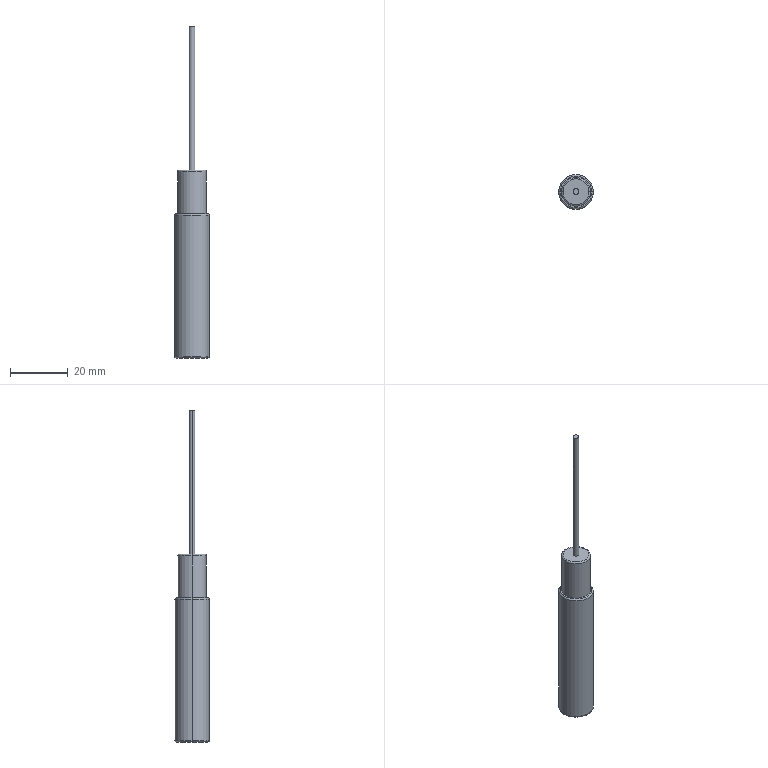Part | STEP file | YB Inductive Proximity Switch | 1 solid | 16 faces | box 12 x 12 x 115 mm | volume 6984 mm3 | torus 6 | cylinder 6 | plane 4 | commonest cylinder face diameters 2 x2 10 x2 12 x2
STEP:
#1=CARTESIAN_POINT('',(0.,0.,0.));
#2=DIRECTION('',(0.,0.,1.));
#3=DIRECTION('',(1.,0.,0.));
#4=AXIS2_PLACEMENT_3D('',#1,#2,#3);
#5=CARTESIAN_POINT('',(-5.5,0.,0.));
#6=VERTEX_POINT('',#5);
#7=CARTESIAN_POINT('',(5.5,0.,0.));
#8=VERTEX_POINT('',#7);
#9=CARTESIAN_POINT('',(0.,0.,0.));
#10=DIRECTION('',(0.,0.,-1.));
#11=DIRECTION('',(1.,0.,0.));
#12=AXIS2_PLACEMENT_3D('',#9,#10,#11);
#13=CIRCLE('',#12,5.5);
#14=CARTESIAN_POINT('',(0.,0.,0.5));
#15=DIRECTION('',(0.,0.,1.));
#16=DIRECTION('',(1.,0.,0.));
#17=AXIS2_PLACEMENT_3D('',#14,#15,#16);
#18=TOROIDAL_SURFACE('',#17,5.5,0.5);
#19=CARTESIAN_POINT('',(6.283,4.712));
#20=DIRECTION('',(-1.,0.));
#21=VECTOR('',#20,1.);
#22=LINE('',#19,#21);
#23=(GEOMETRIC_REPRESENTATION_CONTEXT(2)PARAMETRIC_REPRESENTATION_CONTEXT()REPRESENTATION_CONTEXT('',''));
#24=DEFINITIONAL_REPRESENTATION('',(#22),#23);
#25=PCURVE('',#18,#24);
#26=CARTESIAN_POINT('',(0.,0.,0.));
#27=DIRECTION('',(0.,0.,1.));
#28=DIRECTION('',(1.,0.,0.));
#29=AXIS2_PLACEMENT_3D('',#26,#27,#28);
#30=PLANE('',#29);
#31=CARTESIAN_POINT('',(5.5,0.));
#32=CARTESIAN_POINT('',(5.5,-9.526));
#33=CARTESIAN_POINT('',(-2.75,-4.763));
#34=CARTESIAN_POINT('',(-11.,0.));
#35=CARTESIAN_POINT('',(-2.75,4.763));
#36=CARTESIAN_POINT('',(5.5,9.526));
#37=CARTESIAN_POINT('',(5.5,0.));
#38=(BOUNDED_CURVE()B_SPLINE_CURVE(2,(#31,#32,#33,#34,#35,#36,#37),.UNSPECIFIED.,.T.,.F.)B_SPLINE_CURVE_WITH_KNOTS((1,2,2,2,2,1),(-2.094,0.,2.094,4.189,6.283,8.378),.UNSPECIFIED.)CURVE()GEOMETRIC_REPRESENTATION_ITEM()RATIONAL_B_SPLINE_CURVE((1.,0.5,1.,0.5,1.,0.5,1.))REPRESENTATION_ITEM(''));
#39=(GEOMETRIC_REPRESENTATION_CONTEXT(2)PARAMETRIC_REPRESENTATION_CONTEXT()REPRESENTATION_CONTEXT('',''));
#40=DEFINITIONAL_REPRESENTATION('',(#38),#39);
#41=PCURVE('',#30,#40);
#42=SURFACE_CURVE('',#13,(#25,#41),.PCURVE_S1.);
#43=EDGE_CURVE('',#6,#8,#42,.T.);
#44=ORIENTED_EDGE('',*,*,#43,.F.);
#45=CARTESIAN_POINT('',(-6.,0.,0.5));
#46=VERTEX_POINT('',#45);
#47=CARTESIAN_POINT('',(-5.5,0.,0.5));
#48=DIRECTION('',(0.,1.,0.));
#49=DIRECTION('',(-1.,0.,0.));
#50=AXIS2_PLACEMENT_3D('',#47,#48,#49);
#51=CIRCLE('',#50,0.5);
#52=CARTESIAN_POINT('',(3.142,0.));
#53=DIRECTION('',(0.,1.));
#54=VECTOR('',#53,1.);
#55=LINE('',#52,#54);
#56=(GEOMETRIC_REPRESENTATION_CONTEXT(2)PARAMETRIC_REPRESENTATION_CONTEXT()REPRESENTATION_CONTEXT('',''));
#57=DEFINITIONAL_REPRESENTATION('',(#55),#56);
#58=PCURVE('',#18,#57);
#59=CARTESIAN_POINT('',(0.,0.,0.5));
#60=DIRECTION('',(0.,0.,1.));
#61=DIRECTION('',(1.,0.,0.));
#62=AXIS2_PLACEMENT_3D('',#59,#60,#61);
#63=TOROIDAL_SURFACE('',#62,5.5,0.5);
#64=CARTESIAN_POINT('',(3.142,0.));
#65=DIRECTION('',(0.,1.));
#66=VECTOR('',#65,1.);
#67=LINE('',#64,#66);
#68=(GEOMETRIC_REPRESENTATION_CONTEXT(2)PARAMETRIC_REPRESENTATION_CONTEXT()REPRESENTATION_CONTEXT('',''));
#69=DEFINITIONAL_REPRESENTATION('',(#67),#68);
#70=PCURVE('',#63,#69);
#71=SURFACE_CURVE('',#51,(#58,#70),.PCURVE_S1.);
#72=EDGE_CURVE('',#6,#46,#71,.T.);
#73=ORIENTED_EDGE('',*,*,#72,.T.);
#74=CARTESIAN_POINT('',(6.,0.,0.5));
#75=VERTEX_POINT('',#74);
#76=CARTESIAN_POINT('',(0.,0.,0.5));
#77=DIRECTION('',(0.,0.,1.));
#78=DIRECTION('',(1.,0.,0.));
#79=AXIS2_PLACEMENT_3D('',#76,#77,#78);
#80=CIRCLE('',#79,6.);
#81=CARTESIAN_POINT('',(0.,6.283));
#82=DIRECTION('',(1.,0.));
#83=VECTOR('',#82,1.);
#84=LINE('',#81,#83);
#85=(GEOMETRIC_REPRESENTATION_CONTEXT(2)PARAMETRIC_REPRESENTATION_CONTEXT()REPRESENTATION_CONTEXT('',''));
#86=DEFINITIONAL_REPRESENTATION('',(#84),#85);
#87=PCURVE('',#18,#86);
#88=CARTESIAN_POINT('',(0.,0.,50.));
#89=DIRECTION('',(0.,0.,-1.));
#90=DIRECTION('',(-1.,0.,0.));
#91=AXIS2_PLACEMENT_3D('',#88,#89,#90);
#92=CYLINDRICAL_SURFACE('',#91,6.);
#93=CARTESIAN_POINT('',(3.142,49.5));
#94=DIRECTION('',(-1.,0.));
#95=VECTOR('',#94,1.);
#96=LINE('',#93,#95);
#97=(GEOMETRIC_REPRESENTATION_CONTEXT(2)PARAMETRIC_REPRESENTATION_CONTEXT()REPRESENTATION_CONTEXT('',''));
#98=DEFINITIONAL_REPRESENTATION('',(#96),#97);
#99=PCURVE('',#92,#98);
#100=SURFACE_CURVE('',#80,(#87,#99),.PCURVE_S1.);
#101=EDGE_CURVE('',#75,#46,#100,.T.);
#102=ORIENTED_EDGE('',*,*,#101,.F.);
#103=CARTESIAN_POINT('',(5.5,0.,0.5));
#104=DIRECTION('',(0.,-1.,0.));
#105=DIRECTION('',(0.,0.,-1.));
#106=AXIS2_PLACEMENT_3D('',#103,#104,#105);
#107=CIRCLE('',#106,0.5);
#108=CARTESIAN_POINT('',(0.,4.712));
#109=DIRECTION('',(0.,1.));
#110=VECTOR('',#109,1.);
#111=LINE('',#108,#110);
#112=(GEOMETRIC_REPRESENTATION_CONTEXT(2)PARAMETRIC_REPRESENTATION_CONTEXT()REPRESENTATION_CONTEXT('',''));
#113=DEFINITIONAL_REPRESENTATION('',(#111),#112);
#114=PCURVE('',#18,#113);
#115=CARTESIAN_POINT('',(6.283,4.712));
#116=DIRECTION('',(0.,1.));
#117=VECTOR('',#116,1.);
#118=LINE('',#115,#117);
#119=(GEOMETRIC_REPRESENTATION_CONTEXT(2)PARAMETRIC_REPRESENTATION_CONTEXT()REPRESENTATION_CONTEXT('',''));
#120=DEFINITIONAL_REPRESENTATION('',(#118),#119);
#121=PCURVE('',#63,#120);
#122=SURFACE_CURVE('',#107,(#114,#121),.PCURVE_S1.);
#123=EDGE_CURVE('',#8,#75,#122,.T.);
#124=ORIENTED_EDGE('',*,*,#123,.F.);
#125=EDGE_LOOP('',(#44,#73,#102,#124));
#126=FACE_BOUND('',#125,.T.);
#127=ADVANCED_FACE('',(#126),#18,.T.);
#128=CARTESIAN_POINT('',(-6.,0.,49.5));
#129=VERTEX_POINT('',#128);
#130=CARTESIAN_POINT('',(6.,0.,49.5));
#131=VERTEX_POINT('',#130);
#132=CARTESIAN_POINT('',(0.,0.,49.5));
#133=DIRECTION('',(0.,0.,-1.));
#134=DIRECTION('',(1.,0.,0.));
#135=AXIS2_PLACEMENT_3D('',#132,#133,#134);
#136=CIRCLE('',#135,6.);
#137=CARTESIAN_POINT('',(0.,0.,49.5));
#138=DIRECTION('',(0.,0.,1.));
#139=DIRECTION('',(1.,0.,0.));
#140=AXIS2_PLACEMENT_3D('',#137,#138,#139);
#141=TOROIDAL_SURFACE('',#140,5.5,0.5);
#142=CARTESIAN_POINT('',(6.283,0.));
#143=DIRECTION('',(-1.,0.));
#144=VECTOR('',#143,1.);
#145=LINE('',#142,#144);
#146=(GEOMETRIC_REPRESENTATION_CONTEXT(2)PARAMETRIC_REPRESENTATION_CONTEXT()REPRESENTATION_CONTEXT('',''));
#147=DEFINITIONAL_REPRESENTATION('',(#145),#146);
#148=PCURVE('',#141,#147);
#149=CARTESIAN_POINT('',(-3.142,0.5));
#150=DIRECTION('',(1.,0.));
#151=VECTOR('',#150,1.);
#152=LINE('',#149,#151);
#153=(GEOMETRIC_REPRESENTATION_CONTEXT(2)PARAMETRIC_REPRESENTATION_CONTEXT()REPRESENTATION_CONTEXT('',''));
#154=DEFINITIONAL_REPRESENTATION('',(#152),#153);
#155=PCURVE('',#92,#154);
#156=SURFACE_CURVE('',#136,(#148,#155),.PCURVE_S1.);
#157=EDGE_CURVE('',#129,#131,#156,.T.);
#158=ORIENTED_EDGE('',*,*,#157,.F.);
#159=CARTESIAN_POINT('',(-5.5,0.,50.));
#160=VERTEX_POINT('',#159);
#161=CARTESIAN_POINT('',(-5.5,0.,49.5));
#162=DIRECTION('',(0.,1.,0.));
#163=DIRECTION('',(-1.,0.,0.));
#164=AXIS2_PLACEMENT_3D('',#161,#162,#163);
#165=CIRCLE('',#164,0.5);
#166=CARTESIAN_POINT('',(3.142,0.));
#167=DIRECTION('',(0.,1.));
#168=VECTOR('',#167,1.);
#169=LINE('',#166,#168);
#170=(GEOMETRIC_REPRESENTATION_CONTEXT(2)PARAMETRIC_REPRESENTATION_CONTEXT()REPRESENTATION_CONTEXT('',''));
#171=DEFINITIONAL_REPRESENTATION('',(#169),#170);
#172=PCURVE('',#141,#171);
#173=CARTESIAN_POINT('',(0.,0.,49.5));
#174=DIRECTION('',(0.,0.,1.));
#175=DIRECTION('',(1.,0.,0.));
#176=AXIS2_PLACEMENT_3D('',#173,#174,#175);
#177=TOROIDAL_SURFACE('',#176,5.5,0.5);
#178=CARTESIAN_POINT('',(3.142,0.));
#179=DIRECTION('',(0.,1.));
#180=VECTOR('',#179,1.);
#181=LINE('',#178,#180);
#182=(GEOMETRIC_REPRESENTATION_CONTEXT(2)PARAMETRIC_REPRESENTATION_CONTEXT()REPRESENTATION_CONTEXT('',''));
#183=DEFINITIONAL_REPRESENTATION('',(#181),#182);
#184=PCURVE('',#177,#183);
#185=SURFACE_CURVE('',#165,(#172,#184),.PCURVE_S1.);
#186=EDGE_CURVE('',#129,#160,#185,.T.);
#187=ORIENTED_EDGE('',*,*,#186,.T.);
#188=CARTESIAN_POINT('',(5.5,0.,50.));
#189=VERTEX_POINT('',#188);
#190=CARTESIAN_POINT('',(0.,0.,50.));
#191=DIRECTION('',(0.,0.,1.));
#192=DIRECTION('',(1.,0.,0.));
#193=AXIS2_PLACEMENT_3D('',#190,#191,#192);
#194=CIRCLE('',#193,5.5);
#195=CARTESIAN_POINT('',(0.,1.571));
#196=DIRECTION('',(1.,0.));
#197=VECTOR('',#196,1.);
#198=LINE('',#195,#197);
#199=(GEOMETRIC_REPRESENTATION_CONTEXT(2)PARAMETRIC_REPRESENTATION_CONTEXT()REPRESENTATION_CONTEXT('',''));
#200=DEFINITIONAL_REPRESENTATION('',(#198),#199);
#201=PCURVE('',#141,#200);
#202=CARTESIAN_POINT('',(0.,0.,50.));
#203=DIRECTION('',(0.,0.,1.));
#204=DIRECTION('',(1.,0.,0.));
#205=AXIS2_PLACEMENT_3D('',#202,#203,#204);
#206=PLANE('',#205);
#207=CARTESIAN_POINT('',(0.,0.));
#208=DIRECTION('',(1.,0.));
#209=AXIS2_PLACEMENT_2D('',#207,#208);
#210=CIRCLE('',#209,5.5);
#211=(GEOMETRIC_REPRESENTATION_CONTEXT(2)PARAMETRIC_REPRESENTATION_CONTEXT()REPRESENTATION_CONTEXT('',''));
#212=DEFINITIONAL_REPRESENTATION('',(#210),#211);
#213=PCURVE('',#206,#212);
#214=SURFACE_CURVE('',#194,(#201,#213),.PCURVE_S1.);
#215=EDGE_CURVE('',#189,#160,#214,.T.);
#216=ORIENTED_EDGE('',*,*,#215,.F.);
#217=CARTESIAN_POINT('',(5.5,0.,49.5));
#218=DIRECTION('',(0.,-1.,0.));
#219=DIRECTION('',(0.,0.,-1.));
#220=AXIS2_PLACEMENT_3D('',#217,#218,#219);
#221=CIRCLE('',#220,0.5);
#222=CARTESIAN_POINT('',(0.,-1.571));
#223=DIRECTION('',(0.,1.));
#224=VECTOR('',#223,1.);
#225=LINE('',#222,#224);
#226=(GEOMETRIC_REPRESENTATION_CONTEXT(2)PARAMETRIC_REPRESENTATION_CONTEXT()REPRESENTATION_CONTEXT('',''));
#227=DEFINITIONAL_REPRESENTATION('',(#225),#226);
#228=PCURVE('',#141,#227);
#229=CARTESIAN_POINT('',(6.283,-1.571));
#230=DIRECTION('',(0.,1.));
#231=VECTOR('',#230,1.);
#232=LINE('',#229,#231);
#233=(GEOMETRIC_REPRESENTATION_CONTEXT(2)PARAMETRIC_REPRESENTATION_CONTEXT()REPRESENTATION_CONTEXT('',''));
#234=DEFINITIONAL_REPRESENTATION('',(#232),#233);
#235=PCURVE('',#177,#234);
#236=SURFACE_CURVE('',#221,(#228,#235),.PCURVE_S1.);
#237=EDGE_CURVE('',#131,#189,#236,.T.);
#238=ORIENTED_EDGE('',*,*,#237,.F.);
#239=EDGE_LOOP('',(#158,#187,#216,#238));
#240=FACE_BOUND('',#239,.T.);
#241=ADVANCED_FACE('',(#240),#141,.T.);
#242=CARTESIAN_POINT('',(-5.,0.,64.5));
#243=VERTEX_POINT('',#242);
#244=CARTESIAN_POINT('',(5.,0.,64.5));
#245=VERTEX_POINT('',#244);
#246=CARTESIAN_POINT('',(0.,0.,64.5));
#247=DIRECTION('',(0.,0.,-1.));
#248=DIRECTION('',(1.,0.,0.));
#249=AXIS2_PLACEMENT_3D('',#246,#247,#248);
#250=CIRCLE('',#249,5.);
#251=CARTESIAN_POINT('',(0.,0.,64.5));
#252=DIRECTION('',(0.,0.,1.));
#253=DIRECTION('',(1.,0.,0.));
#254=AXIS2_PLACEMENT_3D('',#251,#252,#253);
#255=TOROIDAL_SURFACE('',#254,4.5,0.5);
#256=CARTESIAN_POINT('',(6.283,0.));
#257=DIRECTION('',(-1.,0.));
#258=VECTOR('',#257,1.);
#259=LINE('',#256,#258);
#260=(GEOMETRIC_REPRESENTATION_CONTEXT(2)PARAMETRIC_REPRESENTATION_CONTEXT()REPRESENTATION_CONTEXT('',''));
#261=DEFINITIONAL_REPRESENTATION('',(#259),#260);
#262=PCURVE('',#255,#261);
#263=CARTESIAN_POINT('',(0.,0.,65.));
#264=DIRECTION('',(0.,0.,-1.));
#265=DIRECTION('',(-1.,0.,0.));
#266=AXIS2_PLACEMENT_3D('',#263,#264,#265);
#267=CYLINDRICAL_SURFACE('',#266,5.);
#268=CARTESIAN_POINT('',(-3.142,0.5));
#269=DIRECTION('',(1.,0.));
#270=VECTOR('',#269,1.);
#271=LINE('',#268,#270);
#272=(GEOMETRIC_REPRESENTATION_CONTEXT(2)PARAMETRIC_REPRESENTATION_CONTEXT()REPRESENTATION_CONTEXT('',''));
#273=DEFINITIONAL_REPRESENTATION('',(#271),#272);
#274=PCURVE('',#267,#273);
#275=SURFACE_CURVE('',#250,(#262,#274),.PCURVE_S1.);
#276=EDGE_CURVE('',#243,#245,#275,.T.);
#277=ORIENTED_EDGE('',*,*,#276,.F.);
#278=CARTESIAN_POINT('',(-4.5,0.,65.));
#279=VERTEX_POINT('',#278);
#280=CARTESIAN_POINT('',(-4.5,0.,64.5));
#281=DIRECTION('',(0.,1.,0.));
#282=DIRECTION('',(-1.,0.,0.));
#283=AXIS2_PLACEMENT_3D('',#280,#281,#282);
#284=CIRCLE('',#283,0.5);
#285=CARTESIAN_POINT('',(3.142,0.));
#286=DIRECTION('',(0.,1.));
#287=VECTOR('',#286,1.);
#288=LINE('',#285,#287);
#289=(GEOMETRIC_REPRESENTATION_CONTEXT(2)PARAMETRIC_REPRESENTATION_CONTEXT()REPRESENTATION_CONTEXT('',''));
#290=DEFINITIONAL_REPRESENTATION('',(#288),#289);
#291=PCURVE('',#255,#290);
#292=CARTESIAN_POINT('',(0.,0.,64.5));
#293=DIRECTION('',(0.,0.,1.));
#294=DIRECTION('',(1.,0.,0.));
#295=AXIS2_PLACEMENT_3D('',#292,#293,#294);
#296=TOROIDAL_SURFACE('',#295,4.5,0.5);
#297=CARTESIAN_POINT('',(3.142,0.));
#298=DIRECTION('',(0.,1.));
#299=VECTOR('',#298,1.);
#300=LINE('',#297,#299);
#301=(GEOMETRIC_REPRESENTATION_CONTEXT(2)PARAMETRIC_REPRESENTATION_CONTEXT()REPRESENTATION_CONTEXT('',''));
#302=DEFINITIONAL_REPRESENTATION('',(#300),#301);
#303=PCURVE('',#296,#302);
#304=SURFACE_CURVE('',#284,(#291,#303),.PCURVE_S1.);
#305=EDGE_CURVE('',#243,#279,#304,.T.);
#306=ORIENTED_EDGE('',*,*,#305,.T.);
#307=CARTESIAN_POINT('',(4.5,0.,65.));
#308=VERTEX_POINT('',#307);
#309=CARTESIAN_POINT('',(0.,0.,65.));
#310=DIRECTION('',(0.,0.,1.));
#311=DIRECTION('',(1.,0.,0.));
#312=AXIS2_PLACEMENT_3D('',#309,#310,#311);
#313=CIRCLE('',#312,4.5);
#314=CARTESIAN_POINT('',(0.,1.571));
#315=DIRECTION('',(1.,0.));
#316=VECTOR('',#315,1.);
#317=LINE('',#314,#316);
#318=(GEOMETRIC_REPRESENTATION_CONTEXT(2)PARAMETRIC_REPRESENTATION_CONTEXT()REPRESENTATION_CONTEXT('',''));
#319=DEFINITIONAL_REPRESENTATION('',(#317),#318);
#320=PCURVE('',#255,#319);
#321=CARTESIAN_POINT('',(0.,0.,65.));
#322=DIRECTION('',(0.,0.,1.));
#323=DIRECTION('',(1.,0.,0.));
#324=AXIS2_PLACEMENT_3D('',#321,#322,#323);
#325=PLANE('',#324);
#326=CARTESIAN_POINT('',(0.,0.));
#327=DIRECTION('',(1.,0.));
#328=AXIS2_PLACEMENT_2D('',#326,#327);
#329=CIRCLE('',#328,4.5);
#330=(GEOMETRIC_REPRESENTATION_CONTEXT(2)PARAMETRIC_REPRESENTATION_CONTEXT()REPRESENTATION_CONTEXT('',''));
#331=DEFINITIONAL_REPRESENTATION('',(#329),#330);
#332=PCURVE('',#325,#331);
#333=SURFACE_CURVE('',#313,(#320,#332),.PCURVE_S1.);
#334=EDGE_CURVE('',#308,#279,#333,.T.);
#335=ORIENTED_EDGE('',*,*,#334,.F.);
#336=CARTESIAN_POINT('',(4.5,0.,64.5));
#337=DIRECTION('',(0.,-1.,0.));
#338=DIRECTION('',(0.,0.,-1.));
#339=AXIS2_PLACEMENT_3D('',#336,#337,#338);
#340=CIRCLE('',#339,0.5);
#341=CARTESIAN_POINT('',(0.,-1.571));
#342=DIRECTION('',(0.,1.));
#343=VECTOR('',#342,1.);
#344=LINE('',#341,#343);
#345=(GEOMETRIC_REPRESENTATION_CONTEXT(2)PARAMETRIC_REPRESENTATION_CONTEXT()REPRESENTATION_CONTEXT('',''));
#346=DEFINITIONAL_REPRESENTATION('',(#344),#345);
#347=PCURVE('',#255,#346);
#348=CARTESIAN_POINT('',(6.283,-1.571));
#349=DIRECTION('',(0.,1.));
#350=VECTOR('',#349,1.);
#351=LINE('',#348,#350);
#352=(GEOMETRIC_REPRESENTATION_CONTEXT(2)PARAMETRIC_REPRESENTATION_CONTEXT()REPRESENTATION_CONTEXT('',''));
#353=DEFINITIONAL_REPRESENTATION('',(#351),#352);
#354=PCURVE('',#296,#353);
#355=SURFACE_CURVE('',#340,(#347,#354),.PCURVE_S1.);
#356=EDGE_CURVE('',#245,#308,#355,.T.);
#357=ORIENTED_EDGE('',*,*,#356,.F.);
#358=EDGE_LOOP('',(#277,#306,#335,#357));
#359=FACE_BOUND('',#358,.T.);
#360=ADVANCED_FACE('',(#359),#255,.T.);
#361=CARTESIAN_POINT('',(1.,0.,115.));
#362=VERTEX_POINT('',#361);
#363=CARTESIAN_POINT('',(-1.,0.,115.));
#364=VERTEX_POINT('',#363);
#365=CARTESIAN_POINT('',(0.,0.,115.));
#366=DIRECTION('',(0.,0.,1.));
#367=DIRECTION('',(1.,0.,0.));
#368=AXIS2_PLACEMENT_3D('',#365,#366,#367);
#369=CIRCLE('',#368,1.);
#370=CARTESIAN_POINT('',(0.,0.,115.));
#371=DIRECTION('',(0.,0.,-1.));
#372=DIRECTION('',(-1.,0.,0.));
#373=AXIS2_PLACEMENT_3D('',#370,#371,#372);
#374=CYLINDRICAL_SURFACE('',#373,1.);
#375=CARTESIAN_POINT('',(3.142,0.));
#376=DIRECTION('',(-1.,0.));
#377=VECTOR('',#376,1.);
#378=LINE('',#375,#377);
#379=(GEOMETRIC_REPRESENTATION_CONTEXT(2)PARAMETRIC_REPRESENTATION_CONTEXT()REPRESENTATION_CONTEXT('',''));
#380=DEFINITIONAL_REPRESENTATION('',(#378),#379);
#381=PCURVE('',#374,#380);
#382=CARTESIAN_POINT('',(0.,0.,115.));
#383=DIRECTION('',(0.,0.,1.));
#384=DIRECTION('',(1.,0.,0.));
#385=AXIS2_PLACEMENT_3D('',#382,#383,#384);
#386=PLANE('',#385);
#387=CARTESIAN_POINT('',(0.,0.));
#388=DIRECTION('',(1.,0.));
#389=AXIS2_PLACEMENT_2D('',#387,#388);
#390=CIRCLE('',#389,1.);
#391=(GEOMETRIC_REPRESENTATION_CONTEXT(2)PARAMETRIC_REPRESENTATION_CONTEXT()REPRESENTATION_CONTEXT('',''));
#392=DEFINITIONAL_REPRESENTATION('',(#390),#391);
#393=PCURVE('',#386,#392);
#394=SURFACE_CURVE('',#369,(#381,#393),.PCURVE_S1.);
#395=EDGE_CURVE('',#362,#364,#394,.T.);
#396=ORIENTED_EDGE('',*,*,#395,.F.);
#397=CARTESIAN_POINT('',(1.,0.,65.));
#398=VERTEX_POINT('',#397);
#399=CARTESIAN_POINT('',(1.,0.,115.));
#400=DIRECTION('',(0.,0.,-1.));
#401=VECTOR('',#400,1.);
#402=LINE('',#399,#401);
#403=CARTESIAN_POINT('',(3.142,0.));
#404=DIRECTION('',(0.,1.));
#405=VECTOR('',#404,1.);
#406=LINE('',#403,#405);
#407=(GEOMETRIC_REPRESENTATION_CONTEXT(2)PARAMETRIC_REPRESENTATION_CONTEXT()REPRESENTATION_CONTEXT('',''));
#408=DEFINITIONAL_REPRESENTATION('',(#406),#407);
#409=PCURVE('',#374,#408);
#410=CARTESIAN_POINT('',(0.,0.,115.));
#411=DIRECTION('',(0.,0.,-1.));
#412=DIRECTION('',(-1.,0.,0.));
#413=AXIS2_PLACEMENT_3D('',#410,#411,#412);
#414=CYLINDRICAL_SURFACE('',#413,1.);
#415=CARTESIAN_POINT('',(3.142,0.));
#416=DIRECTION('',(0.,1.));
#417=VECTOR('',#416,1.);
#418=LINE('',#415,#417);
#419=(GEOMETRIC_REPRESENTATION_CONTEXT(2)PARAMETRIC_REPRESENTATION_CONTEXT()REPRESENTATION_CONTEXT('',''));
#420=DEFINITIONAL_REPRESENTATION('',(#418),#419);
#421=PCURVE('',#414,#420);
#422=SURFACE_CURVE('',#402,(#409,#421),.PCURVE_S1.);
#423=EDGE_CURVE('',#362,#398,#422,.T.);
#424=ORIENTED_EDGE('',*,*,#423,.T.);
#425=CARTESIAN_POINT('',(-1.,0.,65.));
#426=VERTEX_POINT('',#425);
#427=CARTESIAN_POINT('',(0.,0.,65.));
#428=DIRECTION('',(0.,0.,1.));
#429=DIRECTION('',(1.,0.,0.));
#430=AXIS2_PLACEMENT_3D('',#427,#428,#429);
#431=CIRCLE('',#430,1.);
#432=CARTESIAN_POINT('',(3.142,50.));
#433=DIRECTION('',(-1.,0.));
#434=VECTOR('',#433,1.);
#435=LINE('',#432,#434);
#436=(GEOMETRIC_REPRESENTATION_CONTEXT(2)PARAMETRIC_REPRESENTATION_CONTEXT()REPRESENTATION_CONTEXT('',''));
#437=DEFINITIONAL_REPRESENTATION('',(#435),#436);
#438=PCURVE('',#374,#437);
#439=CARTESIAN_POINT('',(0.,0.));
#440=DIRECTION('',(1.,0.));
#441=AXIS2_PLACEMENT_2D('',#439,#440);
#442=CIRCLE('',#441,1.);
#443=(GEOMETRIC_REPRESENTATION_CONTEXT(2)PARAMETRIC_REPRESENTATION_CONTEXT()REPRESENTATION_CONTEXT('',''));
#444=DEFINITIONAL_REPRESENTATION('',(#442),#443);
#445=PCURVE('',#325,#444);
#446=SURFACE_CURVE('',#431,(#438,#445),.PCURVE_S1.);
#447=EDGE_CURVE('',#398,#426,#446,.T.);
#448=ORIENTED_EDGE('',*,*,#447,.T.);
#449=CARTESIAN_POINT('',(-1.,0.,115.));
#450=DIRECTION('',(0.,0.,-1.));
#451=VECTOR('',#450,1.);
#452=LINE('',#449,#451);
#453=CARTESIAN_POINT('',(0.,0.));
#454=DIRECTION('',(0.,1.));
#455=VECTOR('',#454,1.);
#456=LINE('',#453,#455);
#457=(GEOMETRIC_REPRESENTATION_CONTEXT(2)PARAMETRIC_REPRESENTATION_CONTEXT()REPRESENTATION_CONTEXT('',''));
#458=DEFINITIONAL_REPRESENTATION('',(#456),#457);
#459=PCURVE('',#374,#458);
#460=CARTESIAN_POINT('',(6.283,0.));
#461=DIRECTION('',(0.,1.));
#462=VECTOR('',#461,1.);
#463=LINE('',#460,#462);
#464=(GEOMETRIC_REPRESENTATION_CONTEXT(2)PARAMETRIC_REPRESENTATION_CONTEXT()REPRESENTATION_CONTEXT('',''));
#465=DEFINITIONAL_REPRESENTATION('',(#463),#464);
#466=PCURVE('',#414,#465);
#467=SURFACE_CURVE('',#452,(#459,#466),.PCURVE_S1.);
#468=EDGE_CURVE('',#364,#426,#467,.T.);
#469=ORIENTED_EDGE('',*,*,#468,.F.);
#470=EDGE_LOOP('',(#396,#424,#448,#469));
#471=FACE_BOUND('',#470,.T.);
#472=ADVANCED_FACE('',(#471),#374,.T.);
#473=ORIENTED_EDGE('',*,*,#276,.T.);
#474=CARTESIAN_POINT('',(5.,0.,50.));
#475=VERTEX_POINT('',#474);
#476=CARTESIAN_POINT('',(5.,0.,65.));
#477=DIRECTION('',(0.,0.,-1.));
#478=VECTOR('',#477,1.);
#479=LINE('',#476,#478);
#480=CARTESIAN_POINT('',(3.142,0.));
#481=DIRECTION('',(0.,1.));
#482=VECTOR('',#481,1.);
#483=LINE('',#480,#482);
#484=(GEOMETRIC_REPRESENTATION_CONTEXT(2)PARAMETRIC_REPRESENTATION_CONTEXT()REPRESENTATION_CONTEXT('',''));
#485=DEFINITIONAL_REPRESENTATION('',(#483),#484);
#486=PCURVE('',#267,#485);
#487=CARTESIAN_POINT('',(0.,0.,65.));
#488=DIRECTION('',(0.,0.,-1.));
#489=DIRECTION('',(-1.,0.,0.));
#490=AXIS2_PLACEMENT_3D('',#487,#488,#489);
#491=CYLINDRICAL_SURFACE('',#490,5.);
#492=CARTESIAN_POINT('',(3.142,0.));
#493=DIRECTION('',(0.,1.));
#494=VECTOR('',#493,1.);
#495=LINE('',#492,#494);
#496=(GEOMETRIC_REPRESENTATION_CONTEXT(2)PARAMETRIC_REPRESENTATION_CONTEXT()REPRESENTATION_CONTEXT('',''));
#497=DEFINITIONAL_REPRESENTATION('',(#495),#496);
#498=PCURVE('',#491,#497);
#499=SURFACE_CURVE('',#479,(#486,#498),.PCURVE_S1.);
#500=EDGE_CURVE('',#245,#475,#499,.T.);
#501=ORIENTED_EDGE('',*,*,#500,.T.);
#502=CARTESIAN_POINT('',(-5.,0.,50.));
#503=VERTEX_POINT('',#502);
#504=CARTESIAN_POINT('',(0.,0.,50.));
#505=DIRECTION('',(0.,0.,1.));
#506=DIRECTION('',(1.,0.,0.));
#507=AXIS2_PLACEMENT_3D('',#504,#505,#506);
#508=CIRCLE('',#507,5.);
#509=CARTESIAN_POINT('',(3.142,15.));
#510=DIRECTION('',(-1.,0.));
#511=VECTOR('',#510,1.);
#512=LINE('',#509,#511);
#513=(GEOMETRIC_REPRESENTATION_CONTEXT(2)PARAMETRIC_REPRESENTATION_CONTEXT()REPRESENTATION_CONTEXT('',''));
#514=DEFINITIONAL_REPRESENTATION('',(#512),#513);
#515=PCURVE('',#267,#514);
#516=CARTESIAN_POINT('',(0.,0.));
#517=DIRECTION('',(1.,0.));
#518=AXIS2_PLACEMENT_2D('',#516,#517);
#519=CIRCLE('',#518,5.);
#520=(GEOMETRIC_REPRESENTATION_CONTEXT(2)PARAMETRIC_REPRESENTATION_CONTEXT()REPRESENTATION_CONTEXT('',''));
#521=DEFINITIONAL_REPRESENTATION('',(#519),#520);
#522=PCURVE('',#206,#521);
#523=SURFACE_CURVE('',#508,(#515,#522),.PCURVE_S1.);
#524=EDGE_CURVE('',#475,#503,#523,.T.);
#525=ORIENTED_EDGE('',*,*,#524,.T.);
#526=CARTESIAN_POINT('',(-5.,0.,65.));
#527=DIRECTION('',(0.,0.,-1.));
#528=VECTOR('',#527,1.);
#529=LINE('',#526,#528);
#530=CARTESIAN_POINT('',(0.,0.));
#531=DIRECTION('',(0.,1.));
#532=VECTOR('',#531,1.);
#533=LINE('',#530,#532);
#534=(GEOMETRIC_REPRESENTATION_CONTEXT(2)PARAMETRIC_REPRESENTATION_CONTEXT()REPRESENTATION_CONTEXT('',''));
#535=DEFINITIONAL_REPRESENTATION('',(#533),#534);
#536=PCURVE('',#267,#535);
#537=CARTESIAN_POINT('',(6.283,0.));
#538=DIRECTION('',(0.,1.));
#539=VECTOR('',#538,1.);
#540=LINE('',#537,#539);
#541=(GEOMETRIC_REPRESENTATION_CONTEXT(2)PARAMETRIC_REPRESENTATION_CONTEXT()REPRESENTATION_CONTEXT('',''));
#542=DEFINITIONAL_REPRESENTATION('',(#540),#541);
#543=PCURVE('',#491,#542);
#544=SURFACE_CURVE('',#529,(#536,#543),.PCURVE_S1.);
#545=EDGE_CURVE('',#243,#503,#544,.T.);
#546=ORIENTED_EDGE('',*,*,#545,.F.);
#547=EDGE_LOOP('',(#473,#501,#525,#546));
#548=FACE_BOUND('',#547,.T.);
#549=ADVANCED_FACE('',(#548),#267,.T.);
#550=ORIENTED_EDGE('',*,*,#157,.T.);
#551=CARTESIAN_POINT('',(6.,0.,50.));
#552=DIRECTION('',(0.,0.,-1.));
#553=VECTOR('',#552,1.);
#554=LINE('',#551,#553);
#555=CARTESIAN_POINT('',(3.142,0.));
#556=DIRECTION('',(0.,1.));
#557=VECTOR('',#556,1.);
#558=LINE('',#555,#557);
#559=(GEOMETRIC_REPRESENTATION_CONTEXT(2)PARAMETRIC_REPRESENTATION_CONTEXT()REPRESENTATION_CONTEXT('',''));
#560=DEFINITIONAL_REPRESENTATION('',(#558),#559);
#561=PCURVE('',#92,#560);
#562=CARTESIAN_POINT('',(0.,0.,50.));
#563=DIRECTION('',(0.,0.,-1.));
#564=DIRECTION('',(-1.,0.,0.));
#565=AXIS2_PLACEMENT_3D('',#562,#563,#564);
#566=CYLINDRICAL_SURFACE('',#565,6.);
#567=CARTESIAN_POINT('',(3.142,0.));
#568=DIRECTION('',(0.,1.));
#569=VECTOR('',#568,1.);
#570=LINE('',#567,#569);
#571=(GEOMETRIC_REPRESENTATION_CONTEXT(2)PARAMETRIC_REPRESENTATION_CONTEXT()REPRESENTATION_CONTEXT('',''));
#572=DEFINITIONAL_REPRESENTATION('',(#570),#571);
#573=PCURVE('',#566,#572);
#574=SURFACE_CURVE('',#554,(#561,#573),.PCURVE_S1.);
#575=EDGE_CURVE('',#131,#75,#574,.T.);
#576=ORIENTED_EDGE('',*,*,#575,.T.);
#577=ORIENTED_EDGE('',*,*,#101,.T.);
#578=CARTESIAN_POINT('',(-6.,0.,50.));
#579=DIRECTION('',(0.,0.,-1.));
#580=VECTOR('',#579,1.);
#581=LINE('',#578,#580);
#582=CARTESIAN_POINT('',(0.,0.));
#583=DIRECTION('',(0.,1.));
#584=VECTOR('',#583,1.);
#585=LINE('',#582,#584);
#586=(GEOMETRIC_REPRESENTATION_CONTEXT(2)PARAMETRIC_REPRESENTATION_CONTEXT()REPRESENTATION_CONTEXT('',''));
#587=DEFINITIONAL_REPRESENTATION('',(#585),#586);
#588=PCURVE('',#92,#587);
#589=CARTESIAN_POINT('',(6.283,0.));
#590=DIRECTION('',(0.,1.));
#591=VECTOR('',#590,1.);
#592=LINE('',#589,#591);
#593=(GEOMETRIC_REPRESENTATION_CONTEXT(2)PARAMETRIC_REPRESENTATION_CONTEXT()REPRESENTATION_CONTEXT('',''));
#594=DEFINITIONAL_REPRESENTATION('',(#592),#593);
#595=PCURVE('',#566,#594);
#596=SURFACE_CURVE('',#581,(#588,#595),.PCURVE_S1.);
#597=EDGE_CURVE('',#129,#46,#596,.T.);
#598=ORIENTED_EDGE('',*,*,#597,.F.);
#599=EDGE_LOOP('',(#550,#576,#577,#598));
#600=FACE_BOUND('',#599,.T.);
#601=ADVANCED_FACE('',(#600),#92,.T.);
#602=ORIENTED_EDGE('',*,*,#334,.T.);
#603=CARTESIAN_POINT('',(0.,0.,65.));
#604=DIRECTION('',(0.,0.,1.));
#605=DIRECTION('',(1.,0.,0.));
#606=AXIS2_PLACEMENT_3D('',#603,#604,#605);
#607=CIRCLE('',#606,4.5);
#608=CARTESIAN_POINT('',(0.,0.));
#609=DIRECTION('',(1.,0.));
#610=AXIS2_PLACEMENT_2D('',#608,#609);
#611=CIRCLE('',#610,4.5);
#612=(GEOMETRIC_REPRESENTATION_CONTEXT(2)PARAMETRIC_REPRESENTATION_CONTEXT()REPRESENTATION_CONTEXT('',''));
#613=DEFINITIONAL_REPRESENTATION('',(#611),#612);
#614=PCURVE('',#325,#613);
#615=CARTESIAN_POINT('',(0.,1.571));
#616=DIRECTION('',(1.,0.));
#617=VECTOR('',#616,1.);
#618=LINE('',#615,#617);
#619=(GEOMETRIC_REPRESENTATION_CONTEXT(2)PARAMETRIC_REPRESENTATION_CONTEXT()REPRESENTATION_CONTEXT('',''));
#620=DEFINITIONAL_REPRESENTATION('',(#618),#619);
#621=PCURVE('',#296,#620);
#622=SURFACE_CURVE('',#607,(#614,#621),.PCURVE_S1.);
#623=EDGE_CURVE('',#279,#308,#622,.T.);
#624=ORIENTED_EDGE('',*,*,#623,.T.);
#625=EDGE_LOOP('',(#602,#624));
#626=FACE_BOUND('',#625,.T.);
#627=CARTESIAN_POINT('',(0.,0.,65.));
#628=DIRECTION('',(0.,0.,1.));
#629=DIRECTION('',(1.,0.,0.));
#630=AXIS2_PLACEMENT_3D('',#627,#628,#629);
#631=CIRCLE('',#630,1.);
#632=CARTESIAN_POINT('',(0.,0.));
#633=DIRECTION('',(1.,0.));
#634=AXIS2_PLACEMENT_2D('',#632,#633);
#635=CIRCLE('',#634,1.);
#636=(GEOMETRIC_REPRESENTATION_CONTEXT(2)PARAMETRIC_REPRESENTATION_CONTEXT()REPRESENTATION_CONTEXT('',''));
#637=DEFINITIONAL_REPRESENTATION('',(#635),#636);
#638=PCURVE('',#325,#637);
#639=CARTESIAN_POINT('',(9.425,50.));
#640=DIRECTION('',(-1.,0.));
#641=VECTOR('',#640,1.);
#642=LINE('',#639,#641);
#643=(GEOMETRIC_REPRESENTATION_CONTEXT(2)PARAMETRIC_REPRESENTATION_CONTEXT()REPRESENTATION_CONTEXT('',''));
#644=DEFINITIONAL_REPRESENTATION('',(#642),#643);
#645=PCURVE('',#414,#644);
#646=SURFACE_CURVE('',#631,(#638,#645),.PCURVE_S1.);
#647=EDGE_CURVE('',#426,#398,#646,.T.);
#648=ORIENTED_EDGE('',*,*,#647,.F.);
#649=ORIENTED_EDGE('',*,*,#447,.F.);
#650=EDGE_LOOP('',(#648,#649));
#651=FACE_BOUND('',#650,.T.);
#652=ADVANCED_FACE('',(#626,#651),#325,.T.);
#653=ORIENTED_EDGE('',*,*,#215,.T.);
#654=CARTESIAN_POINT('',(0.,0.,50.));
#655=DIRECTION('',(0.,0.,1.));
#656=DIRECTION('',(1.,0.,0.));
#657=AXIS2_PLACEMENT_3D('',#654,#655,#656);
#658=CIRCLE('',#657,5.5);
#659=CARTESIAN_POINT('',(0.,0.));
#660=DIRECTION('',(1.,0.));
#661=AXIS2_PLACEMENT_2D('',#659,#660);
#662=CIRCLE('',#661,5.5);
#663=(GEOMETRIC_REPRESENTATION_CONTEXT(2)PARAMETRIC_REPRESENTATION_CONTEXT()REPRESENTATION_CONTEXT('',''));
#664=DEFINITIONAL_REPRESENTATION('',(#662),#663);
#665=PCURVE('',#206,#664);
#666=CARTESIAN_POINT('',(0.,1.571));
#667=DIRECTION('',(1.,0.));
#668=VECTOR('',#667,1.);
#669=LINE('',#666,#668);
#670=(GEOMETRIC_REPRESENTATION_CONTEXT(2)PARAMETRIC_REPRESENTATION_CONTEXT()REPRESENTATION_CONTEXT('',''));
#671=DEFINITIONAL_REPRESENTATION('',(#669),#670);
#672=PCURVE('',#177,#671);
#673=SURFACE_CURVE('',#658,(#665,#672),.PCURVE_S1.);
#674=EDGE_CURVE('',#160,#189,#673,.T.);
#675=ORIENTED_EDGE('',*,*,#674,.T.);
#676=EDGE_LOOP('',(#653,#675));
#677=FACE_BOUND('',#676,.T.);
#678=CARTESIAN_POINT('',(0.,0.,50.));
#679=DIRECTION('',(0.,0.,1.));
#680=DIRECTION('',(1.,0.,0.));
#681=AXIS2_PLACEMENT_3D('',#678,#679,#680);
#682=CIRCLE('',#681,5.);
#683=CARTESIAN_POINT('',(0.,0.));
#684=DIRECTION('',(1.,0.));
#685=AXIS2_PLACEMENT_2D('',#683,#684);
#686=CIRCLE('',#685,5.);
#687=(GEOMETRIC_REPRESENTATION_CONTEXT(2)PARAMETRIC_REPRESENTATION_CONTEXT()REPRESENTATION_CONTEXT('',''));
#688=DEFINITIONAL_REPRESENTATION('',(#686),#687);
#689=PCURVE('',#206,#688);
#690=CARTESIAN_POINT('',(9.425,15.));
#691=DIRECTION('',(-1.,0.));
#692=VECTOR('',#691,1.);
#693=LINE('',#690,#692);
#694=(GEOMETRIC_REPRESENTATION_CONTEXT(2)PARAMETRIC_REPRESENTATION_CONTEXT()REPRESENTATION_CONTEXT('',''));
#695=DEFINITIONAL_REPRESENTATION('',(#693),#694);
#696=PCURVE('',#491,#695);
#697=SURFACE_CURVE('',#682,(#689,#696),.PCURVE_S1.);
#698=EDGE_CURVE('',#503,#475,#697,.T.);
#699=ORIENTED_EDGE('',*,*,#698,.F.);
#700=ORIENTED_EDGE('',*,*,#524,.F.);
#701=EDGE_LOOP('',(#699,#700));
#702=FACE_BOUND('',#701,.T.);
#703=ADVANCED_FACE('',(#677,#702),#206,.T.);
#704=ORIENTED_EDGE('',*,*,#575,.F.);
#705=CARTESIAN_POINT('',(0.,0.,49.5));
#706=DIRECTION('',(0.,0.,-1.));
#707=DIRECTION('',(1.,0.,0.));
#708=AXIS2_PLACEMENT_3D('',#705,#706,#707);
#709=CIRCLE('',#708,6.);
#710=CARTESIAN_POINT('',(3.142,0.5));
#711=DIRECTION('',(1.,0.));
#712=VECTOR('',#711,1.);
#713=LINE('',#710,#712);
#714=(GEOMETRIC_REPRESENTATION_CONTEXT(2)PARAMETRIC_REPRESENTATION_CONTEXT()REPRESENTATION_CONTEXT('',''));
#715=DEFINITIONAL_REPRESENTATION('',(#713),#714);
#716=PCURVE('',#566,#715);
#717=CARTESIAN_POINT('',(6.283,0.));
#718=DIRECTION('',(-1.,0.));
#719=VECTOR('',#718,1.);
#720=LINE('',#717,#719);
#721=(GEOMETRIC_REPRESENTATION_CONTEXT(2)PARAMETRIC_REPRESENTATION_CONTEXT()REPRESENTATION_CONTEXT('',''));
#722=DEFINITIONAL_REPRESENTATION('',(#720),#721);
#723=PCURVE('',#177,#722);
#724=SURFACE_CURVE('',#709,(#716,#723),.PCURVE_S1.);
#725=EDGE_CURVE('',#131,#129,#724,.T.);
#726=ORIENTED_EDGE('',*,*,#725,.T.);
#727=ORIENTED_EDGE('',*,*,#597,.T.);
#728=CARTESIAN_POINT('',(0.,0.,0.5));
#729=DIRECTION('',(0.,0.,1.));
#730=DIRECTION('',(1.,0.,0.));
#731=AXIS2_PLACEMENT_3D('',#728,#729,#730);
#732=CIRCLE('',#731,6.);
#733=CARTESIAN_POINT('',(9.425,49.5));
#734=DIRECTION('',(-1.,0.));
#735=VECTOR('',#734,1.);
#736=LINE('',#733,#735);
#737=(GEOMETRIC_REPRESENTATION_CONTEXT(2)PARAMETRIC_REPRESENTATION_CONTEXT()REPRESENTATION_CONTEXT('',''));
#738=DEFINITIONAL_REPRESENTATION('',(#736),#737);
#739=PCURVE('',#566,#738);
#740=CARTESIAN_POINT('',(0.,6.283));
#741=DIRECTION('',(1.,0.));
#742=VECTOR('',#741,1.);
#743=LINE('',#740,#742);
#744=(GEOMETRIC_REPRESENTATION_CONTEXT(2)PARAMETRIC_REPRESENTATION_CONTEXT()REPRESENTATION_CONTEXT('',''));
#745=DEFINITIONAL_REPRESENTATION('',(#743),#744);
#746=PCURVE('',#63,#745);
#747=SURFACE_CURVE('',#732,(#739,#746),.PCURVE_S1.);
#748=EDGE_CURVE('',#46,#75,#747,.T.);
#749=ORIENTED_EDGE('',*,*,#748,.T.);
#750=EDGE_LOOP('',(#704,#726,#727,#749));
#751=FACE_BOUND('',#750,.T.);
#752=ADVANCED_FACE('',(#751),#566,.T.);
#753=CARTESIAN_POINT('',(0.,0.,0.));
#754=DIRECTION('',(0.,0.,-1.));
#755=DIRECTION('',(1.,0.,0.));
#756=AXIS2_PLACEMENT_3D('',#753,#754,#755);
#757=CIRCLE('',#756,5.5);
#758=CARTESIAN_POINT('',(5.5,0.));
#759=CARTESIAN_POINT('',(5.5,-9.526));
#760=CARTESIAN_POINT('',(-2.75,-4.763));
#761=CARTESIAN_POINT('',(-11.,0.));
#762=CARTESIAN_POINT('',(-2.75,4.763));
#763=CARTESIAN_POINT('',(5.5,9.526));
#764=CARTESIAN_POINT('',(5.5,0.));
#765=(BOUNDED_CURVE()B_SPLINE_CURVE(2,(#758,#759,#760,#761,#762,#763,#764),.UNSPECIFIED.,.T.,.F.)B_SPLINE_CURVE_WITH_KNOTS((1,2,2,2,2,1),(-2.094,0.,2.094,4.189,6.283,8.378),.UNSPECIFIED.)CURVE()GEOMETRIC_REPRESENTATION_ITEM()RATIONAL_B_SPLINE_CURVE((1.,0.5,1.,0.5,1.,0.5,1.))REPRESENTATION_ITEM(''));
#766=(GEOMETRIC_REPRESENTATION_CONTEXT(2)PARAMETRIC_REPRESENTATION_CONTEXT()REPRESENTATION_CONTEXT('',''));
#767=DEFINITIONAL_REPRESENTATION('',(#765),#766);
#768=PCURVE('',#30,#767);
#769=CARTESIAN_POINT('',(6.283,4.712));
#770=DIRECTION('',(-1.,0.));
#771=VECTOR('',#770,1.);
#772=LINE('',#769,#771);
#773=(GEOMETRIC_REPRESENTATION_CONTEXT(2)PARAMETRIC_REPRESENTATION_CONTEXT()REPRESENTATION_CONTEXT('',''));
#774=DEFINITIONAL_REPRESENTATION('',(#772),#773);
#775=PCURVE('',#63,#774);
#776=SURFACE_CURVE('',#757,(#768,#775),.PCURVE_S1.);
#777=EDGE_CURVE('',#8,#6,#776,.T.);
#778=ORIENTED_EDGE('',*,*,#777,.T.);
#779=ORIENTED_EDGE('',*,*,#43,.T.);
#780=EDGE_LOOP('',(#778,#779));
#781=FACE_BOUND('',#780,.T.);
#782=ADVANCED_FACE('',(#781),#30,.F.);
#783=ORIENTED_EDGE('',*,*,#500,.F.);
#784=CARTESIAN_POINT('',(0.,0.,64.5));
#785=DIRECTION('',(0.,0.,-1.));
#786=DIRECTION('',(1.,0.,0.));
#787=AXIS2_PLACEMENT_3D('',#784,#785,#786);
#788=CIRCLE('',#787,5.);
#789=CARTESIAN_POINT('',(3.142,0.5));
#790=DIRECTION('',(1.,0.));
#791=VECTOR('',#790,1.);
#792=LINE('',#789,#791);
#793=(GEOMETRIC_REPRESENTATION_CONTEXT(2)PARAMETRIC_REPRESENTATION_CONTEXT()REPRESENTATION_CONTEXT('',''));
#794=DEFINITIONAL_REPRESENTATION('',(#792),#793);
#795=PCURVE('',#491,#794);
#796=CARTESIAN_POINT('',(6.283,0.));
#797=DIRECTION('',(-1.,0.));
#798=VECTOR('',#797,1.);
#799=LINE('',#796,#798);
#800=(GEOMETRIC_REPRESENTATION_CONTEXT(2)PARAMETRIC_REPRESENTATION_CONTEXT()REPRESENTATION_CONTEXT('',''));
#801=DEFINITIONAL_REPRESENTATION('',(#799),#800);
#802=PCURVE('',#296,#801);
#803=SURFACE_CURVE('',#788,(#795,#802),.PCURVE_S1.);
#804=EDGE_CURVE('',#245,#243,#803,.T.);
#805=ORIENTED_EDGE('',*,*,#804,.T.);
#806=ORIENTED_EDGE('',*,*,#545,.T.);
#807=ORIENTED_EDGE('',*,*,#698,.T.);
#808=EDGE_LOOP('',(#783,#805,#806,#807));
#809=FACE_BOUND('',#808,.T.);
#810=ADVANCED_FACE('',(#809),#491,.T.);
#811=ORIENTED_EDGE('',*,*,#423,.F.);
#812=CARTESIAN_POINT('',(0.,0.,115.));
#813=DIRECTION('',(0.,0.,1.));
#814=DIRECTION('',(1.,0.,0.));
#815=AXIS2_PLACEMENT_3D('',#812,#813,#814);
#816=CIRCLE('',#815,1.);
#817=CARTESIAN_POINT('',(9.425,0.));
#818=DIRECTION('',(-1.,0.));
#819=VECTOR('',#818,1.);
#820=LINE('',#817,#819);
#821=(GEOMETRIC_REPRESENTATION_CONTEXT(2)PARAMETRIC_REPRESENTATION_CONTEXT()REPRESENTATION_CONTEXT('',''));
#822=DEFINITIONAL_REPRESENTATION('',(#820),#821);
#823=PCURVE('',#414,#822);
#824=CARTESIAN_POINT('',(0.,0.));
#825=DIRECTION('',(1.,0.));
#826=AXIS2_PLACEMENT_2D('',#824,#825);
#827=CIRCLE('',#826,1.);
#828=(GEOMETRIC_REPRESENTATION_CONTEXT(2)PARAMETRIC_REPRESENTATION_CONTEXT()REPRESENTATION_CONTEXT('',''));
#829=DEFINITIONAL_REPRESENTATION('',(#827),#828);
#830=PCURVE('',#386,#829);
#831=SURFACE_CURVE('',#816,(#823,#830),.PCURVE_S1.);
#832=EDGE_CURVE('',#364,#362,#831,.T.);
#833=ORIENTED_EDGE('',*,*,#832,.F.);
#834=ORIENTED_EDGE('',*,*,#468,.T.);
#835=ORIENTED_EDGE('',*,*,#647,.T.);
#836=EDGE_LOOP('',(#811,#833,#834,#835));
#837=FACE_BOUND('',#836,.T.);
#838=ADVANCED_FACE('',(#837),#414,.T.);
#839=ORIENTED_EDGE('',*,*,#832,.T.);
#840=ORIENTED_EDGE('',*,*,#395,.T.);
#841=EDGE_LOOP('',(#839,#840));
#842=FACE_BOUND('',#841,.T.);
#843=ADVANCED_FACE('',(#842),#386,.T.);
#844=ORIENTED_EDGE('',*,*,#305,.F.);
#845=ORIENTED_EDGE('',*,*,#804,.F.);
#846=ORIENTED_EDGE('',*,*,#356,.T.);
#847=ORIENTED_EDGE('',*,*,#623,.F.);
#848=EDGE_LOOP('',(#844,#845,#846,#847));
#849=FACE_BOUND('',#848,.T.);
#850=ADVANCED_FACE('',(#849),#296,.T.);
#851=ORIENTED_EDGE('',*,*,#186,.F.);
#852=ORIENTED_EDGE('',*,*,#725,.F.);
#853=ORIENTED_EDGE('',*,*,#237,.T.);
#854=ORIENTED_EDGE('',*,*,#674,.F.);
#855=EDGE_LOOP('',(#851,#852,#853,#854));
#856=FACE_BOUND('',#855,.T.);
#857=ADVANCED_FACE('',(#856),#177,.T.);
#858=ORIENTED_EDGE('',*,*,#72,.F.);
#859=ORIENTED_EDGE('',*,*,#777,.F.);
#860=ORIENTED_EDGE('',*,*,#123,.T.);
#861=ORIENTED_EDGE('',*,*,#748,.F.);
#862=EDGE_LOOP('',(#858,#859,#860,#861));
#863=FACE_BOUND('',#862,.T.);
#864=ADVANCED_FACE('',(#863),#63,.T.);
#865=CLOSED_SHELL('',(#127,#241,#360,#472,#549,#601,#652,#703,#752,#782,#810,#838,#843,#850,#857,#864));
#866=MANIFOLD_SOLID_BREP('',#865);
#867=(LENGTH_UNIT()NAMED_UNIT(*)SI_UNIT(.MILLI.,.METRE.));
#868=UNCERTAINTY_MEASURE_WITH_UNIT(LENGTH_MEASURE(0.0000001),#867,'','');
#869=(NAMED_UNIT(*)PLANE_ANGLE_UNIT()SI_UNIT($,.RADIAN.));
#870=(NAMED_UNIT(*)SI_UNIT($,.STERADIAN.)SOLID_ANGLE_UNIT());
#871=(GEOMETRIC_REPRESENTATION_CONTEXT(3)GLOBAL_UNCERTAINTY_ASSIGNED_CONTEXT((#868))GLOBAL_UNIT_ASSIGNED_CONTEXT((#867,#869,#870))REPRESENTATION_CONTEXT('',''));
#872=ADVANCED_BREP_SHAPE_REPRESENTATION('',(#4,#866),#871);